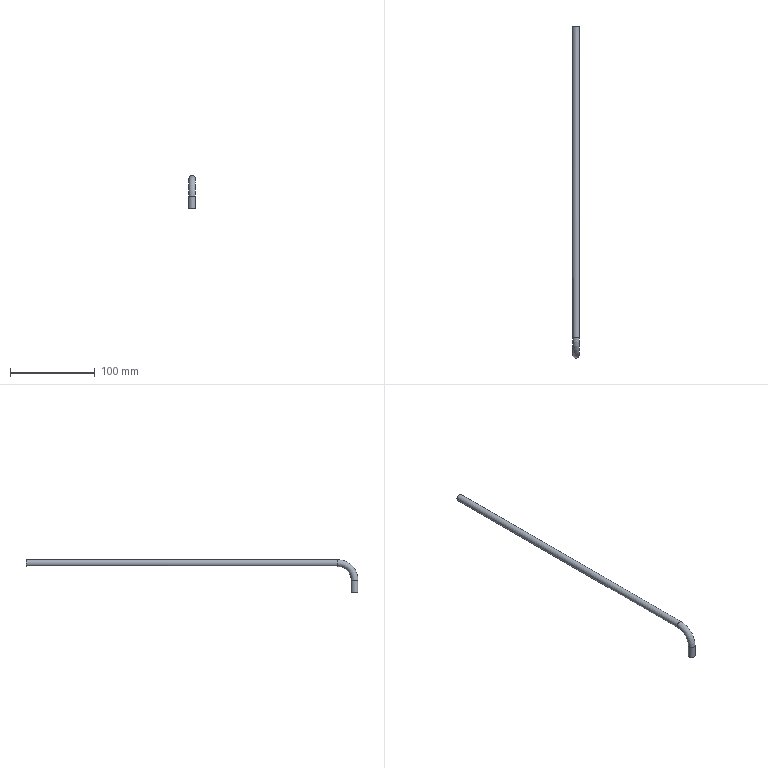Part | STEP file | 1-26.2 | 1 solid | 8 faces | box 8 x 392.074 x 38.526 mm | volume 7072 mm3 | cylinder 4 | torus 2 | plane 2 | commonest cylinder face diameters 6.5 x2 8 x2
STEP:
#1=CARTESIAN_POINT('',(0.,0.,0.));
#2=DIRECTION('',(0.,0.,1.));
#3=DIRECTION('',(1.,0.,0.));
#4=AXIS2_PLACEMENT_3D('',#1,#2,#3);
#5=CARTESIAN_POINT('',(-4.,388.074,0.));
#6=VERTEX_POINT('',#5);
#7=CARTESIAN_POINT('',(0.,388.074,0.));
#8=DIRECTION('',(0.,1.,0.));
#9=DIRECTION('',(-1.,0.,0.));
#10=AXIS2_PLACEMENT_3D('',#7,#8,#9);
#11=CIRCLE('',#10,4.);
#12=CARTESIAN_POINT('',(0.,388.074,0.));
#13=DIRECTION('',(0.,-1.,0.));
#14=DIRECTION('',(-1.,0.,0.));
#15=AXIS2_PLACEMENT_3D('',#12,#13,#14);
#16=CYLINDRICAL_SURFACE('',#15,4.);
#17=CARTESIAN_POINT('',(6.283,0.));
#18=DIRECTION('',(-1.,0.));
#19=VECTOR('',#18,1.);
#20=LINE('',#17,#19);
#21=(GEOMETRIC_REPRESENTATION_CONTEXT(2)PARAMETRIC_REPRESENTATION_CONTEXT()REPRESENTATION_CONTEXT('',''));
#22=DEFINITIONAL_REPRESENTATION('',(#20),#21);
#23=PCURVE('',#16,#22);
#24=CARTESIAN_POINT('',(0.,388.074,0.));
#25=DIRECTION('',(0.,1.,0.));
#26=DIRECTION('',(1.,0.,0.));
#27=AXIS2_PLACEMENT_3D('',#24,#25,#26);
#28=PLANE('',#27);
#29=CARTESIAN_POINT('',(0.,0.));
#30=DIRECTION('',(-1.,0.));
#31=AXIS2_PLACEMENT_2D('',#29,#30);
#32=CIRCLE('',#31,4.);
#33=(GEOMETRIC_REPRESENTATION_CONTEXT(2)PARAMETRIC_REPRESENTATION_CONTEXT()REPRESENTATION_CONTEXT('',''));
#34=DEFINITIONAL_REPRESENTATION('',(#32),#33);
#35=PCURVE('',#28,#34);
#36=SURFACE_CURVE('',#11,(#23,#35),.PCURVE_S1.);
#37=EDGE_CURVE('',#6,#6,#36,.T.);
#38=ORIENTED_EDGE('',*,*,#37,.F.);
#39=CARTESIAN_POINT('',(-4.,20.,0.));
#40=VERTEX_POINT('',#39);
#41=CARTESIAN_POINT('',(-4.,388.074,0.));
#42=DIRECTION('',(0.,-1.,0.));
#43=VECTOR('',#42,1.);
#44=LINE('',#41,#43);
#45=CARTESIAN_POINT('',(6.283,0.));
#46=DIRECTION('',(0.,1.));
#47=VECTOR('',#46,1.);
#48=LINE('',#45,#47);
#49=(GEOMETRIC_REPRESENTATION_CONTEXT(2)PARAMETRIC_REPRESENTATION_CONTEXT()REPRESENTATION_CONTEXT('',''));
#50=DEFINITIONAL_REPRESENTATION('',(#48),#49);
#51=PCURVE('',#16,#50);
#52=CARTESIAN_POINT('',(0.,0.));
#53=DIRECTION('',(0.,1.));
#54=VECTOR('',#53,1.);
#55=LINE('',#52,#54);
#56=(GEOMETRIC_REPRESENTATION_CONTEXT(2)PARAMETRIC_REPRESENTATION_CONTEXT()REPRESENTATION_CONTEXT('',''));
#57=DEFINITIONAL_REPRESENTATION('',(#55),#56);
#58=PCURVE('',#16,#57);
#59=SEAM_CURVE('',#44,(#51,#58),.PCURVE_S1.);
#60=EDGE_CURVE('',#6,#40,#59,.T.);
#61=ORIENTED_EDGE('',*,*,#60,.T.);
#62=CARTESIAN_POINT('',(0.,20.,-4.));
#63=VERTEX_POINT('',#62);
#64=CARTESIAN_POINT('',(0.,20.,0.));
#65=DIRECTION('',(0.,-1.,0.));
#66=DIRECTION('',(0.,0.,-1.));
#67=AXIS2_PLACEMENT_3D('',#64,#65,#66);
#68=CIRCLE('',#67,4.);
#69=CARTESIAN_POINT('',(1.571,368.074));
#70=DIRECTION('',(1.,0.));
#71=VECTOR('',#70,1.);
#72=LINE('',#69,#71);
#73=(GEOMETRIC_REPRESENTATION_CONTEXT(2)PARAMETRIC_REPRESENTATION_CONTEXT()REPRESENTATION_CONTEXT('',''));
#74=DEFINITIONAL_REPRESENTATION('',(#72),#73);
#75=PCURVE('',#16,#74);
#76=CARTESIAN_POINT('',(0.,20.,-20.));
#77=DIRECTION('',(-1.,0.,0.));
#78=DIRECTION('',(0.,0.,1.));
#79=AXIS2_PLACEMENT_3D('',#76,#77,#78);
#80=TOROIDAL_SURFACE('',#79,20.,4.);
#81=CARTESIAN_POINT('',(6.283,3.142));
#82=DIRECTION('',(0.,1.));
#83=VECTOR('',#82,1.);
#84=LINE('',#81,#83);
#85=(GEOMETRIC_REPRESENTATION_CONTEXT(2)PARAMETRIC_REPRESENTATION_CONTEXT()REPRESENTATION_CONTEXT('',''));
#86=DEFINITIONAL_REPRESENTATION('',(#84),#85);
#87=PCURVE('',#80,#86);
#88=SURFACE_CURVE('',#68,(#75,#87),.PCURVE_S1.);
#89=EDGE_CURVE('',#63,#40,#88,.T.);
#90=ORIENTED_EDGE('',*,*,#89,.F.);
#91=CARTESIAN_POINT('',(0.,20.,0.));
#92=DIRECTION('',(0.,-1.,0.));
#93=DIRECTION('',(-1.,0.,0.));
#94=AXIS2_PLACEMENT_3D('',#91,#92,#93);
#95=CIRCLE('',#94,4.);
#96=CARTESIAN_POINT('',(0.,368.074));
#97=DIRECTION('',(1.,0.));
#98=VECTOR('',#97,1.);
#99=LINE('',#96,#98);
#100=(GEOMETRIC_REPRESENTATION_CONTEXT(2)PARAMETRIC_REPRESENTATION_CONTEXT()REPRESENTATION_CONTEXT('',''));
#101=DEFINITIONAL_REPRESENTATION('',(#99),#100);
#102=PCURVE('',#16,#101);
#103=CARTESIAN_POINT('',(6.283,7.854));
#104=DIRECTION('',(0.,1.));
#105=VECTOR('',#104,1.);
#106=LINE('',#103,#105);
#107=(GEOMETRIC_REPRESENTATION_CONTEXT(2)PARAMETRIC_REPRESENTATION_CONTEXT()REPRESENTATION_CONTEXT('',''));
#108=DEFINITIONAL_REPRESENTATION('',(#106),#107);
#109=PCURVE('',#80,#108);
#110=SURFACE_CURVE('',#95,(#102,#109),.PCURVE_S1.);
#111=EDGE_CURVE('',#40,#63,#110,.T.);
#112=ORIENTED_EDGE('',*,*,#111,.F.);
#113=ORIENTED_EDGE('',*,*,#60,.F.);
#114=EDGE_LOOP('',(#38,#61,#90,#112,#113));
#115=FACE_BOUND('',#114,.T.);
#116=ADVANCED_FACE('',(#115),#16,.T.);
#117=ORIENTED_EDGE('',*,*,#89,.T.);
#118=ORIENTED_EDGE('',*,*,#111,.T.);
#119=CARTESIAN_POINT('',(0.,4.,-20.));
#120=VERTEX_POINT('',#119);
#121=CARTESIAN_POINT('',(0.,20.,-20.));
#122=DIRECTION('',(1.,0.,0.));
#123=DIRECTION('',(0.,0.,1.));
#124=AXIS2_PLACEMENT_3D('',#121,#122,#123);
#125=CIRCLE('',#124,16.);
#126=CARTESIAN_POINT('',(6.283,9.425));
#127=DIRECTION('',(-1.,0.));
#128=VECTOR('',#127,1.);
#129=LINE('',#126,#128);
#130=(GEOMETRIC_REPRESENTATION_CONTEXT(2)PARAMETRIC_REPRESENTATION_CONTEXT()REPRESENTATION_CONTEXT('',''));
#131=DEFINITIONAL_REPRESENTATION('',(#129),#130);
#132=PCURVE('',#80,#131);
#133=CARTESIAN_POINT('',(6.283,3.142));
#134=DIRECTION('',(-1.,0.));
#135=VECTOR('',#134,1.);
#136=LINE('',#133,#135);
#137=(GEOMETRIC_REPRESENTATION_CONTEXT(2)PARAMETRIC_REPRESENTATION_CONTEXT()REPRESENTATION_CONTEXT('',''));
#138=DEFINITIONAL_REPRESENTATION('',(#136),#137);
#139=PCURVE('',#80,#138);
#140=SEAM_CURVE('',#125,(#132,#139),.PCURVE_S1.);
#141=EDGE_CURVE('',#63,#120,#140,.T.);
#142=ORIENTED_EDGE('',*,*,#141,.T.);
#143=CARTESIAN_POINT('',(-4.,0.,-20.));
#144=VERTEX_POINT('',#143);
#145=CARTESIAN_POINT('',(0.,0.,-20.));
#146=DIRECTION('',(0.,0.,1.));
#147=DIRECTION('',(0.,1.,0.));
#148=AXIS2_PLACEMENT_3D('',#145,#146,#147);
#149=CIRCLE('',#148,4.);
#150=CARTESIAN_POINT('',(4.712,9.425));
#151=DIRECTION('',(0.,-1.));
#152=VECTOR('',#151,1.);
#153=LINE('',#150,#152);
#154=(GEOMETRIC_REPRESENTATION_CONTEXT(2)PARAMETRIC_REPRESENTATION_CONTEXT()REPRESENTATION_CONTEXT('',''));
#155=DEFINITIONAL_REPRESENTATION('',(#153),#154);
#156=PCURVE('',#80,#155);
#157=CARTESIAN_POINT('',(0.,0.,-20.));
#158=DIRECTION('',(0.,0.,-1.));
#159=DIRECTION('',(-1.,0.,0.));
#160=AXIS2_PLACEMENT_3D('',#157,#158,#159);
#161=CYLINDRICAL_SURFACE('',#160,4.);
#162=CARTESIAN_POINT('',(1.571,0.));
#163=DIRECTION('',(-1.,0.));
#164=VECTOR('',#163,1.);
#165=LINE('',#162,#164);
#166=(GEOMETRIC_REPRESENTATION_CONTEXT(2)PARAMETRIC_REPRESENTATION_CONTEXT()REPRESENTATION_CONTEXT('',''));
#167=DEFINITIONAL_REPRESENTATION('',(#165),#166);
#168=PCURVE('',#161,#167);
#169=SURFACE_CURVE('',#149,(#156,#168),.PCURVE_S1.);
#170=EDGE_CURVE('',#120,#144,#169,.T.);
#171=ORIENTED_EDGE('',*,*,#170,.T.);
#172=CARTESIAN_POINT('',(0.,0.,-20.));
#173=DIRECTION('',(0.,0.,1.));
#174=DIRECTION('',(-1.,0.,0.));
#175=AXIS2_PLACEMENT_3D('',#172,#173,#174);
#176=CIRCLE('',#175,4.);
#177=CARTESIAN_POINT('',(4.712,7.854));
#178=DIRECTION('',(0.,-1.));
#179=VECTOR('',#178,1.);
#180=LINE('',#177,#179);
#181=(GEOMETRIC_REPRESENTATION_CONTEXT(2)PARAMETRIC_REPRESENTATION_CONTEXT()REPRESENTATION_CONTEXT('',''));
#182=DEFINITIONAL_REPRESENTATION('',(#180),#181);
#183=PCURVE('',#80,#182);
#184=CARTESIAN_POINT('',(6.283,0.));
#185=DIRECTION('',(-1.,0.));
#186=VECTOR('',#185,1.);
#187=LINE('',#184,#186);
#188=(GEOMETRIC_REPRESENTATION_CONTEXT(2)PARAMETRIC_REPRESENTATION_CONTEXT()REPRESENTATION_CONTEXT('',''));
#189=DEFINITIONAL_REPRESENTATION('',(#187),#188);
#190=PCURVE('',#161,#189);
#191=SURFACE_CURVE('',#176,(#183,#190),.PCURVE_S1.);
#192=EDGE_CURVE('',#144,#120,#191,.T.);
#193=ORIENTED_EDGE('',*,*,#192,.T.);
#194=ORIENTED_EDGE('',*,*,#141,.F.);
#195=EDGE_LOOP('',(#117,#118,#142,#171,#193,#194));
#196=FACE_BOUND('',#195,.T.);
#197=ADVANCED_FACE('',(#196),#80,.T.);
#198=ORIENTED_EDGE('',*,*,#170,.F.);
#199=ORIENTED_EDGE('',*,*,#192,.F.);
#200=CARTESIAN_POINT('',(-4.,0.,-34.526));
#201=VERTEX_POINT('',#200);
#202=CARTESIAN_POINT('',(-4.,0.,-20.));
#203=DIRECTION('',(0.,0.,-1.));
#204=VECTOR('',#203,1.);
#205=LINE('',#202,#204);
#206=CARTESIAN_POINT('',(6.283,0.));
#207=DIRECTION('',(0.,1.));
#208=VECTOR('',#207,1.);
#209=LINE('',#206,#208);
#210=(GEOMETRIC_REPRESENTATION_CONTEXT(2)PARAMETRIC_REPRESENTATION_CONTEXT()REPRESENTATION_CONTEXT('',''));
#211=DEFINITIONAL_REPRESENTATION('',(#209),#210);
#212=PCURVE('',#161,#211);
#213=CARTESIAN_POINT('',(0.,0.));
#214=DIRECTION('',(0.,1.));
#215=VECTOR('',#214,1.);
#216=LINE('',#213,#215);
#217=(GEOMETRIC_REPRESENTATION_CONTEXT(2)PARAMETRIC_REPRESENTATION_CONTEXT()REPRESENTATION_CONTEXT('',''));
#218=DEFINITIONAL_REPRESENTATION('',(#216),#217);
#219=PCURVE('',#161,#218);
#220=SEAM_CURVE('',#205,(#212,#219),.PCURVE_S1.);
#221=EDGE_CURVE('',#144,#201,#220,.T.);
#222=ORIENTED_EDGE('',*,*,#221,.T.);
#223=CARTESIAN_POINT('',(0.,0.,-34.526));
#224=DIRECTION('',(0.,0.,-1.));
#225=DIRECTION('',(-1.,0.,0.));
#226=AXIS2_PLACEMENT_3D('',#223,#224,#225);
#227=CIRCLE('',#226,4.);
#228=CARTESIAN_POINT('',(0.,14.526));
#229=DIRECTION('',(1.,0.));
#230=VECTOR('',#229,1.);
#231=LINE('',#228,#230);
#232=(GEOMETRIC_REPRESENTATION_CONTEXT(2)PARAMETRIC_REPRESENTATION_CONTEXT()REPRESENTATION_CONTEXT('',''));
#233=DEFINITIONAL_REPRESENTATION('',(#231),#232);
#234=PCURVE('',#161,#233);
#235=CARTESIAN_POINT('',(0.,0.,-34.526));
#236=DIRECTION('',(0.,0.,-1.));
#237=DIRECTION('',(1.,0.,0.));
#238=AXIS2_PLACEMENT_3D('',#235,#236,#237);
#239=PLANE('',#238);
#240=CARTESIAN_POINT('',(0.,0.));
#241=DIRECTION('',(-1.,0.));
#242=AXIS2_PLACEMENT_2D('',#240,#241);
#243=CIRCLE('',#242,4.);
#244=(GEOMETRIC_REPRESENTATION_CONTEXT(2)PARAMETRIC_REPRESENTATION_CONTEXT()REPRESENTATION_CONTEXT('',''));
#245=DEFINITIONAL_REPRESENTATION('',(#243),#244);
#246=PCURVE('',#239,#245);
#247=SURFACE_CURVE('',#227,(#234,#246),.PCURVE_S1.);
#248=EDGE_CURVE('',#201,#201,#247,.T.);
#249=ORIENTED_EDGE('',*,*,#248,.F.);
#250=ORIENTED_EDGE('',*,*,#221,.F.);
#251=EDGE_LOOP('',(#198,#199,#222,#249,#250));
#252=FACE_BOUND('',#251,.T.);
#253=ADVANCED_FACE('',(#252),#161,.T.);
#254=ORIENTED_EDGE('',*,*,#37,.T.);
#255=EDGE_LOOP('',(#254));
#256=FACE_BOUND('',#255,.T.);
#257=CARTESIAN_POINT('',(-3.25,388.074,0.));
#258=VERTEX_POINT('',#257);
#259=CARTESIAN_POINT('',(0.,388.074,0.));
#260=DIRECTION('',(0.,1.,0.));
#261=DIRECTION('',(-1.,0.,0.));
#262=AXIS2_PLACEMENT_3D('',#259,#260,#261);
#263=CIRCLE('',#262,3.25);
#264=CARTESIAN_POINT('',(0.,0.));
#265=DIRECTION('',(-1.,0.));
#266=AXIS2_PLACEMENT_2D('',#264,#265);
#267=CIRCLE('',#266,3.25);
#268=(GEOMETRIC_REPRESENTATION_CONTEXT(2)PARAMETRIC_REPRESENTATION_CONTEXT()REPRESENTATION_CONTEXT('',''));
#269=DEFINITIONAL_REPRESENTATION('',(#267),#268);
#270=PCURVE('',#28,#269);
#271=CARTESIAN_POINT('',(0.,388.074,0.));
#272=DIRECTION('',(0.,-1.,0.));
#273=DIRECTION('',(-1.,0.,0.));
#274=AXIS2_PLACEMENT_3D('',#271,#272,#273);
#275=CYLINDRICAL_SURFACE('',#274,3.25);
#276=CARTESIAN_POINT('',(6.283,0.));
#277=DIRECTION('',(-1.,0.));
#278=VECTOR('',#277,1.);
#279=LINE('',#276,#278);
#280=(GEOMETRIC_REPRESENTATION_CONTEXT(2)PARAMETRIC_REPRESENTATION_CONTEXT()REPRESENTATION_CONTEXT('',''));
#281=DEFINITIONAL_REPRESENTATION('',(#279),#280);
#282=PCURVE('',#275,#281);
#283=SURFACE_CURVE('',#263,(#270,#282),.PCURVE_S1.);
#284=EDGE_CURVE('',#258,#258,#283,.T.);
#285=ORIENTED_EDGE('',*,*,#284,.F.);
#286=EDGE_LOOP('',(#285));
#287=FACE_BOUND('',#286,.T.);
#288=ADVANCED_FACE('',(#256,#287),#28,.T.);
#289=ORIENTED_EDGE('',*,*,#248,.T.);
#290=EDGE_LOOP('',(#289));
#291=FACE_BOUND('',#290,.T.);
#292=CARTESIAN_POINT('',(-3.25,0.,-34.526));
#293=VERTEX_POINT('',#292);
#294=CARTESIAN_POINT('',(0.,0.,-34.526));
#295=DIRECTION('',(0.,0.,-1.));
#296=DIRECTION('',(-1.,0.,0.));
#297=AXIS2_PLACEMENT_3D('',#294,#295,#296);
#298=CIRCLE('',#297,3.25);
#299=CARTESIAN_POINT('',(0.,0.));
#300=DIRECTION('',(-1.,0.));
#301=AXIS2_PLACEMENT_2D('',#299,#300);
#302=CIRCLE('',#301,3.25);
#303=(GEOMETRIC_REPRESENTATION_CONTEXT(2)PARAMETRIC_REPRESENTATION_CONTEXT()REPRESENTATION_CONTEXT('',''));
#304=DEFINITIONAL_REPRESENTATION('',(#302),#303);
#305=PCURVE('',#239,#304);
#306=CARTESIAN_POINT('',(0.,0.,-20.));
#307=DIRECTION('',(0.,0.,-1.));
#308=DIRECTION('',(-1.,0.,0.));
#309=AXIS2_PLACEMENT_3D('',#306,#307,#308);
#310=CYLINDRICAL_SURFACE('',#309,3.25);
#311=CARTESIAN_POINT('',(0.,14.526));
#312=DIRECTION('',(1.,0.));
#313=VECTOR('',#312,1.);
#314=LINE('',#311,#313);
#315=(GEOMETRIC_REPRESENTATION_CONTEXT(2)PARAMETRIC_REPRESENTATION_CONTEXT()REPRESENTATION_CONTEXT('',''));
#316=DEFINITIONAL_REPRESENTATION('',(#314),#315);
#317=PCURVE('',#310,#316);
#318=SURFACE_CURVE('',#298,(#305,#317),.PCURVE_S1.);
#319=EDGE_CURVE('',#293,#293,#318,.T.);
#320=ORIENTED_EDGE('',*,*,#319,.F.);
#321=EDGE_LOOP('',(#320));
#322=FACE_BOUND('',#321,.T.);
#323=ADVANCED_FACE('',(#291,#322),#239,.T.);
#324=ORIENTED_EDGE('',*,*,#284,.F.);
#325=CARTESIAN_POINT('',(-3.25,20.,0.));
#326=VERTEX_POINT('',#325);
#327=CARTESIAN_POINT('',(-3.25,388.074,0.));
#328=DIRECTION('',(0.,-1.,0.));
#329=VECTOR('',#328,1.);
#330=LINE('',#327,#329);
#331=CARTESIAN_POINT('',(6.283,0.));
#332=DIRECTION('',(0.,1.));
#333=VECTOR('',#332,1.);
#334=LINE('',#331,#333);
#335=(GEOMETRIC_REPRESENTATION_CONTEXT(2)PARAMETRIC_REPRESENTATION_CONTEXT()REPRESENTATION_CONTEXT('',''));
#336=DEFINITIONAL_REPRESENTATION('',(#334),#335);
#337=PCURVE('',#275,#336);
#338=CARTESIAN_POINT('',(0.,0.));
#339=DIRECTION('',(0.,1.));
#340=VECTOR('',#339,1.);
#341=LINE('',#338,#340);
#342=(GEOMETRIC_REPRESENTATION_CONTEXT(2)PARAMETRIC_REPRESENTATION_CONTEXT()REPRESENTATION_CONTEXT('',''));
#343=DEFINITIONAL_REPRESENTATION('',(#341),#342);
#344=PCURVE('',#275,#343);
#345=SEAM_CURVE('',#330,(#337,#344),.PCURVE_S1.);
#346=EDGE_CURVE('',#258,#326,#345,.T.);
#347=ORIENTED_EDGE('',*,*,#346,.T.);
#348=CARTESIAN_POINT('',(0.,20.,-3.25));
#349=VERTEX_POINT('',#348);
#350=CARTESIAN_POINT('',(0.,20.,0.));
#351=DIRECTION('',(0.,-1.,0.));
#352=DIRECTION('',(0.,0.,-1.));
#353=AXIS2_PLACEMENT_3D('',#350,#351,#352);
#354=CIRCLE('',#353,3.25);
#355=CARTESIAN_POINT('',(1.571,368.074));
#356=DIRECTION('',(1.,0.));
#357=VECTOR('',#356,1.);
#358=LINE('',#355,#357);
#359=(GEOMETRIC_REPRESENTATION_CONTEXT(2)PARAMETRIC_REPRESENTATION_CONTEXT()REPRESENTATION_CONTEXT('',''));
#360=DEFINITIONAL_REPRESENTATION('',(#358),#359);
#361=PCURVE('',#275,#360);
#362=CARTESIAN_POINT('',(0.,20.,-20.));
#363=DIRECTION('',(-1.,0.,0.));
#364=DIRECTION('',(0.,0.,1.));
#365=AXIS2_PLACEMENT_3D('',#362,#363,#364);
#366=TOROIDAL_SURFACE('',#365,20.,3.25);
#367=CARTESIAN_POINT('',(6.283,-3.142));
#368=DIRECTION('',(0.,1.));
#369=VECTOR('',#368,1.);
#370=LINE('',#367,#369);
#371=(GEOMETRIC_REPRESENTATION_CONTEXT(2)PARAMETRIC_REPRESENTATION_CONTEXT()REPRESENTATION_CONTEXT('',''));
#372=DEFINITIONAL_REPRESENTATION('',(#370),#371);
#373=PCURVE('',#366,#372);
#374=SURFACE_CURVE('',#354,(#361,#373),.PCURVE_S1.);
#375=EDGE_CURVE('',#349,#326,#374,.T.);
#376=ORIENTED_EDGE('',*,*,#375,.F.);
#377=CARTESIAN_POINT('',(0.,20.,0.));
#378=DIRECTION('',(0.,-1.,0.));
#379=DIRECTION('',(-1.,0.,0.));
#380=AXIS2_PLACEMENT_3D('',#377,#378,#379);
#381=CIRCLE('',#380,3.25);
#382=CARTESIAN_POINT('',(0.,368.074));
#383=DIRECTION('',(1.,0.));
#384=VECTOR('',#383,1.);
#385=LINE('',#382,#384);
#386=(GEOMETRIC_REPRESENTATION_CONTEXT(2)PARAMETRIC_REPRESENTATION_CONTEXT()REPRESENTATION_CONTEXT('',''));
#387=DEFINITIONAL_REPRESENTATION('',(#385),#386);
#388=PCURVE('',#275,#387);
#389=CARTESIAN_POINT('',(6.283,1.571));
#390=DIRECTION('',(0.,1.));
#391=VECTOR('',#390,1.);
#392=LINE('',#389,#391);
#393=(GEOMETRIC_REPRESENTATION_CONTEXT(2)PARAMETRIC_REPRESENTATION_CONTEXT()REPRESENTATION_CONTEXT('',''));
#394=DEFINITIONAL_REPRESENTATION('',(#392),#393);
#395=PCURVE('',#366,#394);
#396=SURFACE_CURVE('',#381,(#388,#395),.PCURVE_S1.);
#397=EDGE_CURVE('',#326,#349,#396,.T.);
#398=ORIENTED_EDGE('',*,*,#397,.F.);
#399=ORIENTED_EDGE('',*,*,#346,.F.);
#400=EDGE_LOOP('',(#324,#347,#376,#398,#399));
#401=FACE_BOUND('',#400,.F.);
#402=ADVANCED_FACE('',(#401),#275,.F.);
#403=ORIENTED_EDGE('',*,*,#375,.T.);
#404=ORIENTED_EDGE('',*,*,#397,.T.);
#405=CARTESIAN_POINT('',(0.,3.25,-20.));
#406=VERTEX_POINT('',#405);
#407=CARTESIAN_POINT('',(0.,20.,-20.));
#408=DIRECTION('',(1.,0.,0.));
#409=DIRECTION('',(0.,0.,1.));
#410=AXIS2_PLACEMENT_3D('',#407,#408,#409);
#411=CIRCLE('',#410,16.75);
#412=CARTESIAN_POINT('',(6.283,3.142));
#413=DIRECTION('',(-1.,0.));
#414=VECTOR('',#413,1.);
#415=LINE('',#412,#414);
#416=(GEOMETRIC_REPRESENTATION_CONTEXT(2)PARAMETRIC_REPRESENTATION_CONTEXT()REPRESENTATION_CONTEXT('',''));
#417=DEFINITIONAL_REPRESENTATION('',(#415),#416);
#418=PCURVE('',#366,#417);
#419=CARTESIAN_POINT('',(6.283,-3.142));
#420=DIRECTION('',(-1.,0.));
#421=VECTOR('',#420,1.);
#422=LINE('',#419,#421);
#423=(GEOMETRIC_REPRESENTATION_CONTEXT(2)PARAMETRIC_REPRESENTATION_CONTEXT()REPRESENTATION_CONTEXT('',''));
#424=DEFINITIONAL_REPRESENTATION('',(#422),#423);
#425=PCURVE('',#366,#424);
#426=SEAM_CURVE('',#411,(#418,#425),.PCURVE_S1.);
#427=EDGE_CURVE('',#349,#406,#426,.T.);
#428=ORIENTED_EDGE('',*,*,#427,.T.);
#429=CARTESIAN_POINT('',(-3.25,0.,-20.));
#430=VERTEX_POINT('',#429);
#431=CARTESIAN_POINT('',(0.,0.,-20.));
#432=DIRECTION('',(0.,0.,1.));
#433=DIRECTION('',(0.,1.,0.));
#434=AXIS2_PLACEMENT_3D('',#431,#432,#433);
#435=CIRCLE('',#434,3.25);
#436=CARTESIAN_POINT('',(4.712,3.142));
#437=DIRECTION('',(0.,-1.));
#438=VECTOR('',#437,1.);
#439=LINE('',#436,#438);
#440=(GEOMETRIC_REPRESENTATION_CONTEXT(2)PARAMETRIC_REPRESENTATION_CONTEXT()REPRESENTATION_CONTEXT('',''));
#441=DEFINITIONAL_REPRESENTATION('',(#439),#440);
#442=PCURVE('',#366,#441);
#443=CARTESIAN_POINT('',(1.571,0.));
#444=DIRECTION('',(-1.,0.));
#445=VECTOR('',#444,1.);
#446=LINE('',#443,#445);
#447=(GEOMETRIC_REPRESENTATION_CONTEXT(2)PARAMETRIC_REPRESENTATION_CONTEXT()REPRESENTATION_CONTEXT('',''));
#448=DEFINITIONAL_REPRESENTATION('',(#446),#447);
#449=PCURVE('',#310,#448);
#450=SURFACE_CURVE('',#435,(#442,#449),.PCURVE_S1.);
#451=EDGE_CURVE('',#406,#430,#450,.T.);
#452=ORIENTED_EDGE('',*,*,#451,.T.);
#453=CARTESIAN_POINT('',(0.,0.,-20.));
#454=DIRECTION('',(0.,0.,1.));
#455=DIRECTION('',(-1.,0.,0.));
#456=AXIS2_PLACEMENT_3D('',#453,#454,#455);
#457=CIRCLE('',#456,3.25);
#458=CARTESIAN_POINT('',(4.712,1.571));
#459=DIRECTION('',(0.,-1.));
#460=VECTOR('',#459,1.);
#461=LINE('',#458,#460);
#462=(GEOMETRIC_REPRESENTATION_CONTEXT(2)PARAMETRIC_REPRESENTATION_CONTEXT()REPRESENTATION_CONTEXT('',''));
#463=DEFINITIONAL_REPRESENTATION('',(#461),#462);
#464=PCURVE('',#366,#463);
#465=CARTESIAN_POINT('',(6.283,0.));
#466=DIRECTION('',(-1.,0.));
#467=VECTOR('',#466,1.);
#468=LINE('',#465,#467);
#469=(GEOMETRIC_REPRESENTATION_CONTEXT(2)PARAMETRIC_REPRESENTATION_CONTEXT()REPRESENTATION_CONTEXT('',''));
#470=DEFINITIONAL_REPRESENTATION('',(#468),#469);
#471=PCURVE('',#310,#470);
#472=SURFACE_CURVE('',#457,(#464,#471),.PCURVE_S1.);
#473=EDGE_CURVE('',#430,#406,#472,.T.);
#474=ORIENTED_EDGE('',*,*,#473,.T.);
#475=ORIENTED_EDGE('',*,*,#427,.F.);
#476=EDGE_LOOP('',(#403,#404,#428,#452,#474,#475));
#477=FACE_BOUND('',#476,.F.);
#478=ADVANCED_FACE('',(#477),#366,.F.);
#479=ORIENTED_EDGE('',*,*,#451,.F.);
#480=ORIENTED_EDGE('',*,*,#473,.F.);
#481=CARTESIAN_POINT('',(-3.25,0.,-20.));
#482=DIRECTION('',(0.,0.,-1.));
#483=VECTOR('',#482,1.);
#484=LINE('',#481,#483);
#485=CARTESIAN_POINT('',(6.283,0.));
#486=DIRECTION('',(0.,1.));
#487=VECTOR('',#486,1.);
#488=LINE('',#485,#487);
#489=(GEOMETRIC_REPRESENTATION_CONTEXT(2)PARAMETRIC_REPRESENTATION_CONTEXT()REPRESENTATION_CONTEXT('',''));
#490=DEFINITIONAL_REPRESENTATION('',(#488),#489);
#491=PCURVE('',#310,#490);
#492=CARTESIAN_POINT('',(0.,0.));
#493=DIRECTION('',(0.,1.));
#494=VECTOR('',#493,1.);
#495=LINE('',#492,#494);
#496=(GEOMETRIC_REPRESENTATION_CONTEXT(2)PARAMETRIC_REPRESENTATION_CONTEXT()REPRESENTATION_CONTEXT('',''));
#497=DEFINITIONAL_REPRESENTATION('',(#495),#496);
#498=PCURVE('',#310,#497);
#499=SEAM_CURVE('',#484,(#491,#498),.PCURVE_S1.);
#500=EDGE_CURVE('',#430,#293,#499,.T.);
#501=ORIENTED_EDGE('',*,*,#500,.T.);
#502=ORIENTED_EDGE('',*,*,#319,.F.);
#503=ORIENTED_EDGE('',*,*,#500,.F.);
#504=EDGE_LOOP('',(#479,#480,#501,#502,#503));
#505=FACE_BOUND('',#504,.F.);
#506=ADVANCED_FACE('',(#505),#310,.F.);
#507=CLOSED_SHELL('',(#116,#197,#253,#288,#323,#402,#478,#506));
#508=MANIFOLD_SOLID_BREP('',#507);
#509=(LENGTH_UNIT()NAMED_UNIT(*)SI_UNIT(.MILLI.,.METRE.));
#510=UNCERTAINTY_MEASURE_WITH_UNIT(LENGTH_MEASURE(0.0000001),#509,'','');
#511=(NAMED_UNIT(*)PLANE_ANGLE_UNIT()SI_UNIT($,.RADIAN.));
#512=(NAMED_UNIT(*)SI_UNIT($,.STERADIAN.)SOLID_ANGLE_UNIT());
#513=(GEOMETRIC_REPRESENTATION_CONTEXT(3)GLOBAL_UNCERTAINTY_ASSIGNED_CONTEXT((#510))GLOBAL_UNIT_ASSIGNED_CONTEXT((#509,#511,#512))REPRESENTATION_CONTEXT('',''));
#514=ADVANCED_BREP_SHAPE_REPRESENTATION('',(#4,#508),#513);